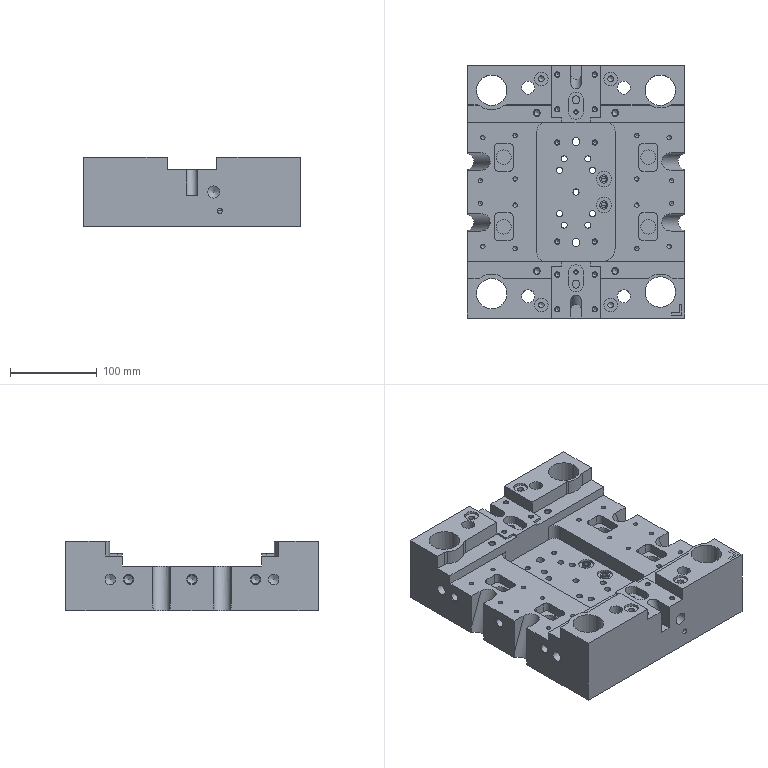Part | STEP file | BB_id58_x_t | 1 solid | 342 faces | box 250 x 290 x 80 mm | volume 3575390 mm3 | cylinder 141 | plane 123 | cone 78 | commonest cylinder face diameters 5 x28 10 x24 7 x9 6.8 x8 17 x8 20 x7